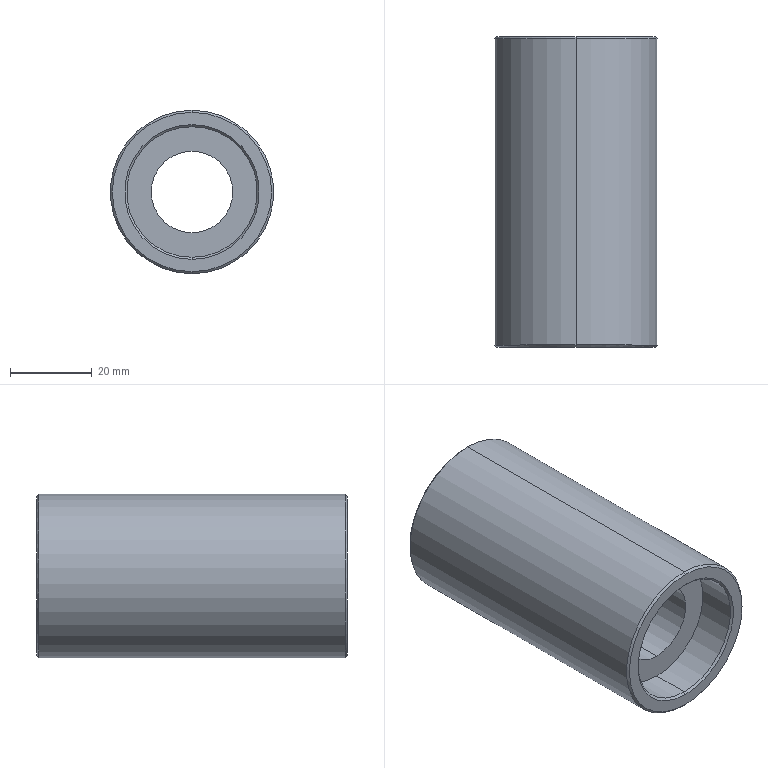Part | STEP file | 10000020449swp000-1 | 1 solid | 20 faces | box 40 x 76 x 40 mm | volume 61770 mm3 | cone 8 | cylinder 8 | plane 4 | commonest cylinder face diameters 32 x4 20 x2 40 x2
STEP:
#1=CARTESIAN_POINT('',(0.,0.,-19.5));
#2=VERTEX_POINT('',#1);
#3=CARTESIAN_POINT('',(0.,0.,19.5));
#4=VERTEX_POINT('',#3);
#5=CARTESIAN_POINT('',(0.,0.,0.));
#6=DIRECTION('',(0.,-1.,0.));
#7=DIRECTION('',(0.,0.,1.));
#8=AXIS2_PLACEMENT_3D('',#5,#6,#7);
#9=CIRCLE('',#8,19.5);
#10=EDGE_CURVE('',#2,#4,#9,.T.);
#11=ORIENTED_EDGE('',*,*,#10,.F.);
#12=CARTESIAN_POINT('',(0.,0.5,-20.));
#13=VERTEX_POINT('',#12);
#14=CARTESIAN_POINT('',(0.,0.5,-20.));
#15=DIRECTION('',(0.,0.7071,-0.7071));
#16=VECTOR('',#15,1000.);
#17=LINE('',#14,#16);
#18=EDGE_CURVE('',#2,#13,#17,.T.);
#19=ORIENTED_EDGE('',*,*,#18,.T.);
#20=CARTESIAN_POINT('',(0.,0.5,20.));
#21=VERTEX_POINT('',#20);
#22=CARTESIAN_POINT('',(0.,0.5,0.));
#23=DIRECTION('',(0.,1.,0.));
#24=DIRECTION('',(0.,0.,1.));
#25=AXIS2_PLACEMENT_3D('',#22,#23,#24);
#26=CIRCLE('',#25,20.);
#27=EDGE_CURVE('',#21,#13,#26,.T.);
#28=ORIENTED_EDGE('',*,*,#27,.F.);
#29=CARTESIAN_POINT('',(0.,0.5,20.));
#30=DIRECTION('',(0.,0.7071,0.7071));
#31=VECTOR('',#30,1000.);
#32=LINE('',#29,#31);
#33=EDGE_CURVE('',#4,#21,#32,.T.);
#34=ORIENTED_EDGE('',*,*,#33,.F.);
#35=EDGE_LOOP('',(#11,#19,#28,#34));
#36=FACE_OUTER_BOUND('',#35,.T.);
#37=CARTESIAN_POINT('',(0.,0.5,0.));
#38=DIRECTION('',(0.,1.,0.));
#39=DIRECTION('',(0.,0.,1.));
#40=AXIS2_PLACEMENT_3D('',#37,#38,#39);
#41=CONICAL_SURFACE('',#40,20.,0.7854);
#42=ADVANCED_FACE('',(#36),#41,.T.);
#43=CARTESIAN_POINT('',(0.,76.,19.5));
#44=VERTEX_POINT('',#43);
#45=CARTESIAN_POINT('',(0.,76.,-19.5));
#46=VERTEX_POINT('',#45);
#47=CARTESIAN_POINT('',(0.,76.,0.));
#48=DIRECTION('',(0.,1.,0.));
#49=DIRECTION('',(0.,0.,1.));
#50=AXIS2_PLACEMENT_3D('',#47,#48,#49);
#51=CIRCLE('',#50,19.5);
#52=EDGE_CURVE('',#44,#46,#51,.T.);
#53=ORIENTED_EDGE('',*,*,#52,.F.);
#54=CARTESIAN_POINT('',(0.,75.5,20.));
#55=VERTEX_POINT('',#54);
#56=CARTESIAN_POINT('',(0.,76.,19.5));
#57=DIRECTION('',(0.,-0.7071,0.7071));
#58=VECTOR('',#57,1000.);
#59=LINE('',#56,#58);
#60=EDGE_CURVE('',#44,#55,#59,.T.);
#61=ORIENTED_EDGE('',*,*,#60,.T.);
#62=CARTESIAN_POINT('',(0.,75.5,-20.));
#63=VERTEX_POINT('',#62);
#64=CARTESIAN_POINT('',(0.,75.5,0.));
#65=DIRECTION('',(0.,-1.,0.));
#66=DIRECTION('',(0.,0.,1.));
#67=AXIS2_PLACEMENT_3D('',#64,#65,#66);
#68=CIRCLE('',#67,20.);
#69=EDGE_CURVE('',#63,#55,#68,.T.);
#70=ORIENTED_EDGE('',*,*,#69,.F.);
#71=CARTESIAN_POINT('',(0.,76.,-19.5));
#72=DIRECTION('',(0.,-0.7071,-0.7071));
#73=VECTOR('',#72,1000.);
#74=LINE('',#71,#73);
#75=EDGE_CURVE('',#46,#63,#74,.T.);
#76=ORIENTED_EDGE('',*,*,#75,.F.);
#77=EDGE_LOOP('',(#53,#61,#70,#76));
#78=FACE_OUTER_BOUND('',#77,.T.);
#79=CARTESIAN_POINT('',(0.,76.,0.));
#80=DIRECTION('',(0.,-1.,0.));
#81=DIRECTION('',(0.,0.,-1.));
#82=AXIS2_PLACEMENT_3D('',#79,#80,#81);
#83=CONICAL_SURFACE('',#82,19.5,0.7854);
#84=ADVANCED_FACE('',(#78),#83,.T.);
#85=CARTESIAN_POINT('',(0.,0.5,16.));
#86=VERTEX_POINT('',#85);
#87=CARTESIAN_POINT('',(0.,0.5,-16.));
#88=VERTEX_POINT('',#87);
#89=CARTESIAN_POINT('',(0.,0.5,0.));
#90=DIRECTION('',(0.,-1.,0.));
#91=DIRECTION('',(0.,0.,1.));
#92=AXIS2_PLACEMENT_3D('',#89,#90,#91);
#93=CIRCLE('',#92,16.);
#94=EDGE_CURVE('',#86,#88,#93,.T.);
#95=ORIENTED_EDGE('',*,*,#94,.F.);
#96=CARTESIAN_POINT('',(0.,0.,16.5));
#97=VERTEX_POINT('',#96);
#98=CARTESIAN_POINT('',(0.,0.5,16.));
#99=DIRECTION('',(0.,-0.7071,0.7071));
#100=VECTOR('',#99,1000.);
#101=LINE('',#98,#100);
#102=EDGE_CURVE('',#86,#97,#101,.T.);
#103=ORIENTED_EDGE('',*,*,#102,.T.);
#104=CARTESIAN_POINT('',(0.,0.,-16.5));
#105=VERTEX_POINT('',#104);
#106=CARTESIAN_POINT('',(0.,0.,0.));
#107=DIRECTION('',(0.,1.,0.));
#108=DIRECTION('',(0.,0.,1.));
#109=AXIS2_PLACEMENT_3D('',#106,#107,#108);
#110=CIRCLE('',#109,16.5);
#111=EDGE_CURVE('',#105,#97,#110,.T.);
#112=ORIENTED_EDGE('',*,*,#111,.F.);
#113=CARTESIAN_POINT('',(0.,0.5,-16.));
#114=DIRECTION('',(0.,-0.7071,-0.7071));
#115=VECTOR('',#114,1000.);
#116=LINE('',#113,#115);
#117=EDGE_CURVE('',#88,#105,#116,.T.);
#118=ORIENTED_EDGE('',*,*,#117,.F.);
#119=EDGE_LOOP('',(#95,#103,#112,#118));
#120=FACE_OUTER_BOUND('',#119,.T.);
#121=CARTESIAN_POINT('',(0.,0.5,0.));
#122=DIRECTION('',(0.,-1.,0.));
#123=DIRECTION('',(0.,0.,-1.));
#124=AXIS2_PLACEMENT_3D('',#121,#122,#123);
#125=CONICAL_SURFACE('',#124,16.,0.7854);
#126=ADVANCED_FACE('',(#120),#125,.F.);
#127=CARTESIAN_POINT('',(0.,75.5,-16.));
#128=VERTEX_POINT('',#127);
#129=CARTESIAN_POINT('',(0.,75.5,16.));
#130=VERTEX_POINT('',#129);
#131=CARTESIAN_POINT('',(0.,75.5,0.));
#132=DIRECTION('',(0.,1.,0.));
#133=DIRECTION('',(0.,0.,1.));
#134=AXIS2_PLACEMENT_3D('',#131,#132,#133);
#135=CIRCLE('',#134,16.);
#136=EDGE_CURVE('',#128,#130,#135,.T.);
#137=ORIENTED_EDGE('',*,*,#136,.F.);
#138=CARTESIAN_POINT('',(0.,76.,-16.5));
#139=VERTEX_POINT('',#138);
#140=CARTESIAN_POINT('',(0.,75.5,-16.));
#141=DIRECTION('',(0.,0.7071,-0.7071));
#142=VECTOR('',#141,1000.);
#143=LINE('',#140,#142);
#144=EDGE_CURVE('',#128,#139,#143,.T.);
#145=ORIENTED_EDGE('',*,*,#144,.T.);
#146=CARTESIAN_POINT('',(0.,76.,16.5));
#147=VERTEX_POINT('',#146);
#148=CARTESIAN_POINT('',(0.,76.,0.));
#149=DIRECTION('',(0.,-1.,0.));
#150=DIRECTION('',(0.,0.,1.));
#151=AXIS2_PLACEMENT_3D('',#148,#149,#150);
#152=CIRCLE('',#151,16.5);
#153=EDGE_CURVE('',#147,#139,#152,.T.);
#154=ORIENTED_EDGE('',*,*,#153,.F.);
#155=CARTESIAN_POINT('',(0.,75.5,16.));
#156=DIRECTION('',(0.,0.7071,0.7071));
#157=VECTOR('',#156,1000.);
#158=LINE('',#155,#157);
#159=EDGE_CURVE('',#130,#147,#158,.T.);
#160=ORIENTED_EDGE('',*,*,#159,.F.);
#161=EDGE_LOOP('',(#137,#145,#154,#160));
#162=FACE_OUTER_BOUND('',#161,.T.);
#163=CARTESIAN_POINT('',(0.,75.5,0.));
#164=DIRECTION('',(0.,1.,0.));
#165=DIRECTION('',(0.,0.,1.));
#166=AXIS2_PLACEMENT_3D('',#163,#164,#165);
#167=CONICAL_SURFACE('',#166,16.,0.7854);
#168=ADVANCED_FACE('',(#162),#167,.F.);
#169=CARTESIAN_POINT('',(0.,66.,-16.));
#170=VERTEX_POINT('',#169);
#171=CARTESIAN_POINT('',(0.,66.,16.));
#172=VERTEX_POINT('',#171);
#173=CARTESIAN_POINT('',(0.,66.,0.));
#174=DIRECTION('',(0.,1.,0.));
#175=DIRECTION('',(0.,0.,1.));
#176=AXIS2_PLACEMENT_3D('',#173,#174,#175);
#177=CIRCLE('',#176,16.);
#178=EDGE_CURVE('',#170,#172,#177,.T.);
#179=ORIENTED_EDGE('',*,*,#178,.F.);
#180=CARTESIAN_POINT('',(0.,76.,-16.));
#181=DIRECTION('',(0.,1.,0.));
#182=VECTOR('',#181,1000.);
#183=LINE('',#180,#182);
#184=EDGE_CURVE('',#170,#128,#183,.T.);
#185=ORIENTED_EDGE('',*,*,#184,.T.);
#186=ORIENTED_EDGE('',*,*,#136,.T.);
#187=CARTESIAN_POINT('',(0.,76.,16.));
#188=DIRECTION('',(0.,1.,0.));
#189=VECTOR('',#188,1000.);
#190=LINE('',#187,#189);
#191=EDGE_CURVE('',#172,#130,#190,.T.);
#192=ORIENTED_EDGE('',*,*,#191,.F.);
#193=EDGE_LOOP('',(#179,#185,#186,#192));
#194=FACE_OUTER_BOUND('',#193,.T.);
#195=CARTESIAN_POINT('',(0.,76.,0.));
#196=DIRECTION('',(0.,1.,0.));
#197=DIRECTION('',(0.,0.,1.));
#198=AXIS2_PLACEMENT_3D('',#195,#196,#197);
#199=CYLINDRICAL_SURFACE('',#198,16.);
#200=ADVANCED_FACE('',(#194),#199,.F.);
#201=CARTESIAN_POINT('',(0.,10.,16.));
#202=VERTEX_POINT('',#201);
#203=CARTESIAN_POINT('',(0.,10.,-16.));
#204=VERTEX_POINT('',#203);
#205=CARTESIAN_POINT('',(0.,10.,0.));
#206=DIRECTION('',(0.,-1.,0.));
#207=DIRECTION('',(0.,0.,-1.));
#208=AXIS2_PLACEMENT_3D('',#205,#206,#207);
#209=CIRCLE('',#208,16.);
#210=EDGE_CURVE('',#202,#204,#209,.T.);
#211=ORIENTED_EDGE('',*,*,#210,.F.);
#212=CARTESIAN_POINT('',(0.,0.,16.));
#213=DIRECTION('',(0.,-1.,0.));
#214=VECTOR('',#213,1000.);
#215=LINE('',#212,#214);
#216=EDGE_CURVE('',#202,#86,#215,.T.);
#217=ORIENTED_EDGE('',*,*,#216,.T.);
#218=ORIENTED_EDGE('',*,*,#94,.T.);
#219=CARTESIAN_POINT('',(0.,0.,-16.));
#220=DIRECTION('',(0.,-1.,0.));
#221=VECTOR('',#220,1000.);
#222=LINE('',#219,#221);
#223=EDGE_CURVE('',#204,#88,#222,.T.);
#224=ORIENTED_EDGE('',*,*,#223,.F.);
#225=EDGE_LOOP('',(#211,#217,#218,#224));
#226=FACE_OUTER_BOUND('',#225,.T.);
#227=CARTESIAN_POINT('',(0.,0.,0.));
#228=DIRECTION('',(0.,-1.,0.));
#229=DIRECTION('',(0.,0.,-1.));
#230=AXIS2_PLACEMENT_3D('',#227,#228,#229);
#231=CYLINDRICAL_SURFACE('',#230,16.);
#232=ADVANCED_FACE('',(#226),#231,.F.);
#233=CARTESIAN_POINT('',(0.,66.,10.));
#234=VERTEX_POINT('',#233);
#235=CARTESIAN_POINT('',(0.,66.,-10.));
#236=VERTEX_POINT('',#235);
#237=CARTESIAN_POINT('',(0.,66.,0.));
#238=DIRECTION('',(0.,-1.,0.));
#239=DIRECTION('',(0.,0.,-1.));
#240=AXIS2_PLACEMENT_3D('',#237,#238,#239);
#241=CIRCLE('',#240,10.);
#242=EDGE_CURVE('',#234,#236,#241,.T.);
#243=ORIENTED_EDGE('',*,*,#242,.F.);
#244=CARTESIAN_POINT('',(0.,10.,10.));
#245=VERTEX_POINT('',#244);
#246=CARTESIAN_POINT('',(0.,76.,10.));
#247=DIRECTION('',(0.,-1.,0.));
#248=VECTOR('',#247,1000.);
#249=LINE('',#246,#248);
#250=EDGE_CURVE('',#234,#245,#249,.T.);
#251=ORIENTED_EDGE('',*,*,#250,.T.);
#252=CARTESIAN_POINT('',(0.,10.,-10.));
#253=VERTEX_POINT('',#252);
#254=CARTESIAN_POINT('',(0.,10.,0.));
#255=DIRECTION('',(0.,1.,0.));
#256=DIRECTION('',(0.,0.,1.));
#257=AXIS2_PLACEMENT_3D('',#254,#255,#256);
#258=CIRCLE('',#257,10.);
#259=EDGE_CURVE('',#253,#245,#258,.T.);
#260=ORIENTED_EDGE('',*,*,#259,.F.);
#261=CARTESIAN_POINT('',(0.,76.,-10.));
#262=DIRECTION('',(0.,-1.,0.));
#263=VECTOR('',#262,1000.);
#264=LINE('',#261,#263);
#265=EDGE_CURVE('',#236,#253,#264,.T.);
#266=ORIENTED_EDGE('',*,*,#265,.F.);
#267=EDGE_LOOP('',(#243,#251,#260,#266));
#268=FACE_OUTER_BOUND('',#267,.T.);
#269=CARTESIAN_POINT('',(0.,76.,0.));
#270=DIRECTION('',(0.,-1.,0.));
#271=DIRECTION('',(0.,0.,-1.));
#272=AXIS2_PLACEMENT_3D('',#269,#270,#271);
#273=CYLINDRICAL_SURFACE('',#272,10.);
#274=ADVANCED_FACE('',(#268),#273,.F.);
#275=ORIENTED_EDGE('',*,*,#69,.T.);
#276=CARTESIAN_POINT('',(0.,76.,20.));
#277=DIRECTION('',(0.,-1.,0.));
#278=VECTOR('',#277,1000.);
#279=LINE('',#276,#278);
#280=EDGE_CURVE('',#55,#21,#279,.T.);
#281=ORIENTED_EDGE('',*,*,#280,.T.);
#282=ORIENTED_EDGE('',*,*,#27,.T.);
#283=CARTESIAN_POINT('',(0.,76.,-20.));
#284=DIRECTION('',(0.,-1.,0.));
#285=VECTOR('',#284,1000.);
#286=LINE('',#283,#285);
#287=EDGE_CURVE('',#63,#13,#286,.T.);
#288=ORIENTED_EDGE('',*,*,#287,.F.);
#289=EDGE_LOOP('',(#275,#281,#282,#288));
#290=FACE_OUTER_BOUND('',#289,.T.);
#291=CARTESIAN_POINT('',(0.,76.,0.));
#292=DIRECTION('',(0.,-1.,0.));
#293=DIRECTION('',(0.,0.,-1.));
#294=AXIS2_PLACEMENT_3D('',#291,#292,#293);
#295=CYLINDRICAL_SURFACE('',#294,20.);
#296=ADVANCED_FACE('',(#290),#295,.T.);
#297=ORIENTED_EDGE('',*,*,#153,.T.);
#298=CARTESIAN_POINT('',(0.,76.,0.));
#299=DIRECTION('',(0.,-1.,0.));
#300=DIRECTION('',(0.,0.,1.));
#301=AXIS2_PLACEMENT_3D('',#298,#299,#300);
#302=CIRCLE('',#301,16.5);
#303=EDGE_CURVE('',#139,#147,#302,.T.);
#304=ORIENTED_EDGE('',*,*,#303,.T.);
#305=EDGE_LOOP('',(#297,#304));
#306=FACE_BOUND('',#305,.T.);
#307=CARTESIAN_POINT('',(0.,76.,0.));
#308=DIRECTION('',(0.,1.,0.));
#309=DIRECTION('',(0.,0.,1.));
#310=AXIS2_PLACEMENT_3D('',#307,#308,#309);
#311=CIRCLE('',#310,19.5);
#312=EDGE_CURVE('',#46,#44,#311,.T.);
#313=ORIENTED_EDGE('',*,*,#312,.T.);
#314=ORIENTED_EDGE('',*,*,#52,.T.);
#315=EDGE_LOOP('',(#313,#314));
#316=FACE_OUTER_BOUND('',#315,.T.);
#317=CARTESIAN_POINT('',(0.,76.,0.));
#318=DIRECTION('',(0.,1.,0.));
#319=DIRECTION('',(0.,0.,1.));
#320=AXIS2_PLACEMENT_3D('',#317,#318,#319);
#321=PLANE('',#320);
#322=ADVANCED_FACE('',(#306,#316),#321,.T.);
#323=ORIENTED_EDGE('',*,*,#111,.T.);
#324=CARTESIAN_POINT('',(0.,0.,0.));
#325=DIRECTION('',(0.,1.,0.));
#326=DIRECTION('',(0.,0.,1.));
#327=AXIS2_PLACEMENT_3D('',#324,#325,#326);
#328=CIRCLE('',#327,16.5);
#329=EDGE_CURVE('',#97,#105,#328,.T.);
#330=ORIENTED_EDGE('',*,*,#329,.T.);
#331=EDGE_LOOP('',(#323,#330));
#332=FACE_BOUND('',#331,.T.);
#333=CARTESIAN_POINT('',(0.,0.,0.));
#334=DIRECTION('',(0.,-1.,0.));
#335=DIRECTION('',(0.,0.,1.));
#336=AXIS2_PLACEMENT_3D('',#333,#334,#335);
#337=CIRCLE('',#336,19.5);
#338=EDGE_CURVE('',#4,#2,#337,.T.);
#339=ORIENTED_EDGE('',*,*,#338,.T.);
#340=ORIENTED_EDGE('',*,*,#10,.T.);
#341=EDGE_LOOP('',(#339,#340));
#342=FACE_OUTER_BOUND('',#341,.T.);
#343=CARTESIAN_POINT('',(0.,0.,0.));
#344=DIRECTION('',(0.,1.,0.));
#345=DIRECTION('',(0.,0.,1.));
#346=AXIS2_PLACEMENT_3D('',#343,#344,#345);
#347=PLANE('',#346);
#348=ADVANCED_FACE('',(#332,#342),#347,.F.);
#349=ORIENTED_EDGE('',*,*,#280,.F.);
#350=CARTESIAN_POINT('',(0.,75.5,0.));
#351=DIRECTION('',(0.,-1.,0.));
#352=DIRECTION('',(0.,0.,1.));
#353=AXIS2_PLACEMENT_3D('',#350,#351,#352);
#354=CIRCLE('',#353,20.);
#355=EDGE_CURVE('',#55,#63,#354,.T.);
#356=ORIENTED_EDGE('',*,*,#355,.T.);
#357=ORIENTED_EDGE('',*,*,#287,.T.);
#358=CARTESIAN_POINT('',(0.,0.5,0.));
#359=DIRECTION('',(0.,1.,0.));
#360=DIRECTION('',(0.,0.,1.));
#361=AXIS2_PLACEMENT_3D('',#358,#359,#360);
#362=CIRCLE('',#361,20.);
#363=EDGE_CURVE('',#13,#21,#362,.T.);
#364=ORIENTED_EDGE('',*,*,#363,.T.);
#365=EDGE_LOOP('',(#349,#356,#357,#364));
#366=FACE_OUTER_BOUND('',#365,.T.);
#367=CARTESIAN_POINT('',(0.,76.,0.));
#368=DIRECTION('',(0.,-1.,0.));
#369=DIRECTION('',(0.,0.,-1.));
#370=AXIS2_PLACEMENT_3D('',#367,#368,#369);
#371=CYLINDRICAL_SURFACE('',#370,20.);
#372=ADVANCED_FACE('',(#366),#371,.T.);
#373=ORIENTED_EDGE('',*,*,#250,.F.);
#374=CARTESIAN_POINT('',(0.,66.,0.));
#375=DIRECTION('',(0.,-1.,0.));
#376=DIRECTION('',(0.,0.,-1.));
#377=AXIS2_PLACEMENT_3D('',#374,#375,#376);
#378=CIRCLE('',#377,10.);
#379=EDGE_CURVE('',#236,#234,#378,.T.);
#380=ORIENTED_EDGE('',*,*,#379,.F.);
#381=ORIENTED_EDGE('',*,*,#265,.T.);
#382=CARTESIAN_POINT('',(0.,10.,0.));
#383=DIRECTION('',(0.,1.,0.));
#384=DIRECTION('',(0.,0.,1.));
#385=AXIS2_PLACEMENT_3D('',#382,#383,#384);
#386=CIRCLE('',#385,10.);
#387=EDGE_CURVE('',#245,#253,#386,.T.);
#388=ORIENTED_EDGE('',*,*,#387,.F.);
#389=EDGE_LOOP('',(#373,#380,#381,#388));
#390=FACE_OUTER_BOUND('',#389,.T.);
#391=CARTESIAN_POINT('',(0.,76.,0.));
#392=DIRECTION('',(0.,-1.,0.));
#393=DIRECTION('',(0.,0.,-1.));
#394=AXIS2_PLACEMENT_3D('',#391,#392,#393);
#395=CYLINDRICAL_SURFACE('',#394,10.);
#396=ADVANCED_FACE('',(#390),#395,.F.);
#397=ORIENTED_EDGE('',*,*,#259,.T.);
#398=ORIENTED_EDGE('',*,*,#387,.T.);
#399=EDGE_LOOP('',(#397,#398));
#400=FACE_BOUND('',#399,.T.);
#401=CARTESIAN_POINT('',(0.,10.,0.));
#402=DIRECTION('',(0.,-1.,0.));
#403=DIRECTION('',(0.,0.,-1.));
#404=AXIS2_PLACEMENT_3D('',#401,#402,#403);
#405=CIRCLE('',#404,16.);
#406=EDGE_CURVE('',#204,#202,#405,.T.);
#407=ORIENTED_EDGE('',*,*,#406,.T.);
#408=ORIENTED_EDGE('',*,*,#210,.T.);
#409=EDGE_LOOP('',(#407,#408));
#410=FACE_OUTER_BOUND('',#409,.T.);
#411=CARTESIAN_POINT('',(0.,10.,0.));
#412=DIRECTION('',(0.,1.,0.));
#413=DIRECTION('',(0.,0.,1.));
#414=AXIS2_PLACEMENT_3D('',#411,#412,#413);
#415=PLANE('',#414);
#416=ADVANCED_FACE('',(#400,#410),#415,.F.);
#417=ORIENTED_EDGE('',*,*,#216,.F.);
#418=ORIENTED_EDGE('',*,*,#406,.F.);
#419=ORIENTED_EDGE('',*,*,#223,.T.);
#420=CARTESIAN_POINT('',(0.,0.5,0.));
#421=DIRECTION('',(0.,-1.,0.));
#422=DIRECTION('',(0.,0.,1.));
#423=AXIS2_PLACEMENT_3D('',#420,#421,#422);
#424=CIRCLE('',#423,16.);
#425=EDGE_CURVE('',#88,#86,#424,.T.);
#426=ORIENTED_EDGE('',*,*,#425,.T.);
#427=EDGE_LOOP('',(#417,#418,#419,#426));
#428=FACE_OUTER_BOUND('',#427,.T.);
#429=CARTESIAN_POINT('',(0.,0.,0.));
#430=DIRECTION('',(0.,-1.,0.));
#431=DIRECTION('',(0.,0.,-1.));
#432=AXIS2_PLACEMENT_3D('',#429,#430,#431);
#433=CYLINDRICAL_SURFACE('',#432,16.);
#434=ADVANCED_FACE('',(#428),#433,.F.);
#435=ORIENTED_EDGE('',*,*,#379,.T.);
#436=ORIENTED_EDGE('',*,*,#242,.T.);
#437=EDGE_LOOP('',(#435,#436));
#438=FACE_BOUND('',#437,.T.);
#439=CARTESIAN_POINT('',(0.,66.,0.));
#440=DIRECTION('',(0.,1.,0.));
#441=DIRECTION('',(0.,0.,1.));
#442=AXIS2_PLACEMENT_3D('',#439,#440,#441);
#443=CIRCLE('',#442,16.);
#444=EDGE_CURVE('',#172,#170,#443,.T.);
#445=ORIENTED_EDGE('',*,*,#444,.T.);
#446=ORIENTED_EDGE('',*,*,#178,.T.);
#447=EDGE_LOOP('',(#445,#446));
#448=FACE_OUTER_BOUND('',#447,.T.);
#449=CARTESIAN_POINT('',(0.,66.,0.));
#450=DIRECTION('',(0.,-1.,0.));
#451=DIRECTION('',(0.,0.,-1.));
#452=AXIS2_PLACEMENT_3D('',#449,#450,#451);
#453=PLANE('',#452);
#454=ADVANCED_FACE('',(#438,#448),#453,.F.);
#455=ORIENTED_EDGE('',*,*,#184,.F.);
#456=ORIENTED_EDGE('',*,*,#444,.F.);
#457=ORIENTED_EDGE('',*,*,#191,.T.);
#458=CARTESIAN_POINT('',(0.,75.5,0.));
#459=DIRECTION('',(0.,1.,0.));
#460=DIRECTION('',(0.,0.,1.));
#461=AXIS2_PLACEMENT_3D('',#458,#459,#460);
#462=CIRCLE('',#461,16.);
#463=EDGE_CURVE('',#130,#128,#462,.T.);
#464=ORIENTED_EDGE('',*,*,#463,.T.);
#465=EDGE_LOOP('',(#455,#456,#457,#464));
#466=FACE_OUTER_BOUND('',#465,.T.);
#467=CARTESIAN_POINT('',(0.,76.,0.));
#468=DIRECTION('',(0.,1.,0.));
#469=DIRECTION('',(0.,0.,1.));
#470=AXIS2_PLACEMENT_3D('',#467,#468,#469);
#471=CYLINDRICAL_SURFACE('',#470,16.);
#472=ADVANCED_FACE('',(#466),#471,.F.);
#473=ORIENTED_EDGE('',*,*,#144,.F.);
#474=ORIENTED_EDGE('',*,*,#463,.F.);
#475=ORIENTED_EDGE('',*,*,#159,.T.);
#476=ORIENTED_EDGE('',*,*,#303,.F.);
#477=EDGE_LOOP('',(#473,#474,#475,#476));
#478=FACE_OUTER_BOUND('',#477,.T.);
#479=CARTESIAN_POINT('',(0.,75.5,0.));
#480=DIRECTION('',(0.,1.,0.));
#481=DIRECTION('',(0.,0.,1.));
#482=AXIS2_PLACEMENT_3D('',#479,#480,#481);
#483=CONICAL_SURFACE('',#482,16.,0.7854);
#484=ADVANCED_FACE('',(#478),#483,.F.);
#485=ORIENTED_EDGE('',*,*,#102,.F.);
#486=ORIENTED_EDGE('',*,*,#425,.F.);
#487=ORIENTED_EDGE('',*,*,#117,.T.);
#488=ORIENTED_EDGE('',*,*,#329,.F.);
#489=EDGE_LOOP('',(#485,#486,#487,#488));
#490=FACE_OUTER_BOUND('',#489,.T.);
#491=CARTESIAN_POINT('',(0.,0.5,0.));
#492=DIRECTION('',(0.,-1.,0.));
#493=DIRECTION('',(0.,0.,-1.));
#494=AXIS2_PLACEMENT_3D('',#491,#492,#493);
#495=CONICAL_SURFACE('',#494,16.,0.7854);
#496=ADVANCED_FACE('',(#490),#495,.F.);
#497=ORIENTED_EDGE('',*,*,#60,.F.);
#498=ORIENTED_EDGE('',*,*,#312,.F.);
#499=ORIENTED_EDGE('',*,*,#75,.T.);
#500=ORIENTED_EDGE('',*,*,#355,.F.);
#501=EDGE_LOOP('',(#497,#498,#499,#500));
#502=FACE_OUTER_BOUND('',#501,.T.);
#503=CARTESIAN_POINT('',(0.,76.,0.));
#504=DIRECTION('',(0.,-1.,0.));
#505=DIRECTION('',(0.,0.,-1.));
#506=AXIS2_PLACEMENT_3D('',#503,#504,#505);
#507=CONICAL_SURFACE('',#506,19.5,0.7854);
#508=ADVANCED_FACE('',(#502),#507,.T.);
#509=ORIENTED_EDGE('',*,*,#18,.F.);
#510=ORIENTED_EDGE('',*,*,#338,.F.);
#511=ORIENTED_EDGE('',*,*,#33,.T.);
#512=ORIENTED_EDGE('',*,*,#363,.F.);
#513=EDGE_LOOP('',(#509,#510,#511,#512));
#514=FACE_OUTER_BOUND('',#513,.T.);
#515=CARTESIAN_POINT('',(0.,0.5,0.));
#516=DIRECTION('',(0.,1.,0.));
#517=DIRECTION('',(0.,0.,1.));
#518=AXIS2_PLACEMENT_3D('',#515,#516,#517);
#519=CONICAL_SURFACE('',#518,20.,0.7854);
#520=ADVANCED_FACE('',(#514),#519,.T.);
#521=CLOSED_SHELL('',(#42,#84,#126,#168,#200,#232,#274,#296,#322,#348,#372,#396,#416,#434,#454,#472,#484,#496,#508,#520));
#522=MANIFOLD_SOLID_BREP('',#521);
#523=CARTESIAN_POINT('',(0.,0.,0.));
#524=DIRECTION('',(0.,0.,1.));
#525=DIRECTION('',(1.,0.,0.));
#526=AXIS2_PLACEMENT_3D('',#523,#524,#525);
#527=(LENGTH_UNIT()NAMED_UNIT(*)SI_UNIT(.MILLI.,.METRE.));
#528=UNCERTAINTY_MEASURE_WITH_UNIT(LENGTH_MEASURE(0.00001),#527,'','');
#529=(NAMED_UNIT(*)PLANE_ANGLE_UNIT()SI_UNIT($,.RADIAN.));
#530=(NAMED_UNIT(*)SI_UNIT($,.STERADIAN.)SOLID_ANGLE_UNIT());
#531=(GEOMETRIC_REPRESENTATION_CONTEXT(3)GLOBAL_UNCERTAINTY_ASSIGNED_CONTEXT((#528))GLOBAL_UNIT_ASSIGNED_CONTEXT((#527,#529,#530))REPRESENTATION_CONTEXT('',''));
#532=ADVANCED_BREP_SHAPE_REPRESENTATION('',(#522,#526),#531);